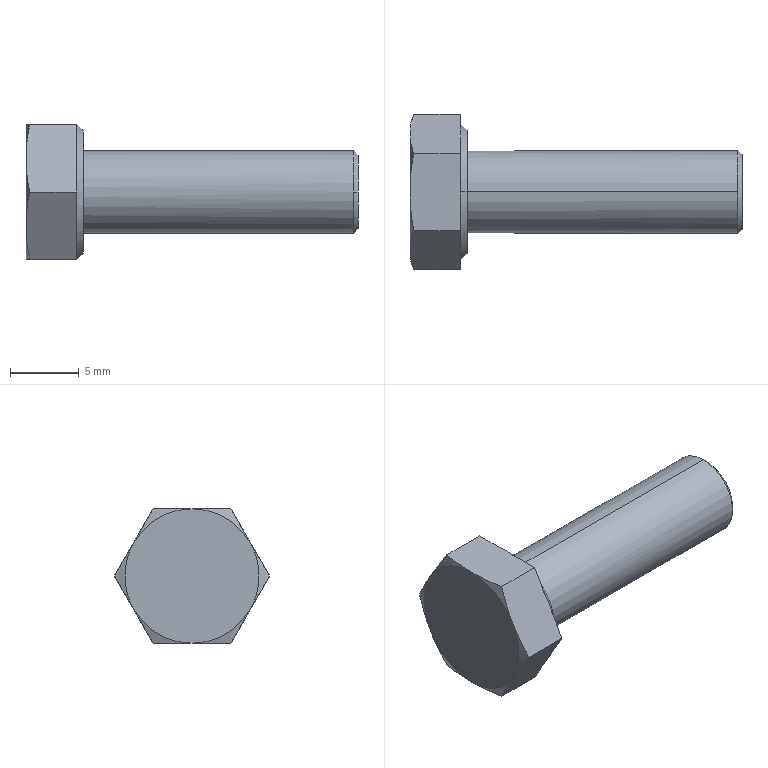Part | NX | features BREP 1 | 1 solid | 27 faces | box 24.15 x 11.293 x 9.78 mm | volume 900.954 mm3 | plane 15 | cone 10 | cylinder 2 | commonest cylinder face diameters 6 x2
STEP:
#1=CARTESIAN_POINT('',(0.,-4.235,-2.445));
#2=VERTEX_POINT('',#1);
#3=CARTESIAN_POINT('',(0.,0.,-4.89));
#4=VERTEX_POINT('',#3);
#5=CARTESIAN_POINT('',(0.,0.,0.));
#6=DIRECTION('',(1.,0.,0.));
#7=DIRECTION('',(0.,0.,-1.));
#8=AXIS2_PLACEMENT_3D('',#5,#6,#7);
#9=CIRCLE('',#8,4.89);
#10=EDGE_CURVE('',#2,#4,#9,.T.);
#11=ORIENTED_EDGE('',*,*,#10,.F.);
#12=CARTESIAN_POINT('',(0.,-4.235,2.445));
#13=VERTEX_POINT('',#12);
#14=CARTESIAN_POINT('',(0.,0.,0.));
#15=DIRECTION('',(1.,0.,0.));
#16=DIRECTION('',(0.,0.,-1.));
#17=AXIS2_PLACEMENT_3D('',#14,#15,#16);
#18=CIRCLE('',#17,4.89);
#19=EDGE_CURVE('',#13,#2,#18,.T.);
#20=ORIENTED_EDGE('',*,*,#19,.F.);
#21=CARTESIAN_POINT('',(0.,0.,4.89));
#22=VERTEX_POINT('',#21);
#23=CARTESIAN_POINT('',(0.,0.,0.));
#24=DIRECTION('',(1.,0.,0.));
#25=DIRECTION('',(0.,0.,-1.));
#26=AXIS2_PLACEMENT_3D('',#23,#24,#25);
#27=CIRCLE('',#26,4.89);
#28=EDGE_CURVE('',#22,#13,#27,.T.);
#29=ORIENTED_EDGE('',*,*,#28,.F.);
#30=CARTESIAN_POINT('',(0.,4.235,2.445));
#31=VERTEX_POINT('',#30);
#32=CARTESIAN_POINT('',(0.,0.,0.));
#33=DIRECTION('',(1.,0.,0.));
#34=DIRECTION('',(0.,0.,-1.));
#35=AXIS2_PLACEMENT_3D('',#32,#33,#34);
#36=CIRCLE('',#35,4.89);
#37=EDGE_CURVE('',#31,#22,#36,.T.);
#38=ORIENTED_EDGE('',*,*,#37,.F.);
#39=CARTESIAN_POINT('',(0.,4.235,-2.445));
#40=VERTEX_POINT('',#39);
#41=CARTESIAN_POINT('',(0.,0.,0.));
#42=DIRECTION('',(1.,0.,0.));
#43=DIRECTION('',(0.,0.,-1.));
#44=AXIS2_PLACEMENT_3D('',#41,#42,#43);
#45=CIRCLE('',#44,4.89);
#46=EDGE_CURVE('',#40,#31,#45,.T.);
#47=ORIENTED_EDGE('',*,*,#46,.F.);
#48=CARTESIAN_POINT('',(0.,0.,0.));
#49=DIRECTION('',(1.,0.,0.));
#50=DIRECTION('',(0.,0.,-1.));
#51=AXIS2_PLACEMENT_3D('',#48,#49,#50);
#52=CIRCLE('',#51,4.89);
#53=EDGE_CURVE('',#4,#40,#52,.T.);
#54=ORIENTED_EDGE('',*,*,#53,.F.);
#55=EDGE_LOOP('',(#11,#20,#29,#38,#47,#54));
#56=FACE_BOUND('',#55,.T.);
#57=CARTESIAN_POINT('',(0.,-2.823,-4.89));
#58=DIRECTION('',(1.,0.,0.));
#59=DIRECTION('',(0.,0.,-1.));
#60=AXIS2_PLACEMENT_3D('',#57,#58,#59);
#61=PLANE('',#60);
#62=ADVANCED_FACE('',(#56),#61,.F.);
#63=ORIENTED_EDGE('',*,*,#46,.T.);
#64=CARTESIAN_POINT('',(0.2753,5.646,0.));
#65=VERTEX_POINT('',#64);
#66=CARTESIAN_POINT('',(0.2753,5.646,0.));
#67=CARTESIAN_POINT('',(0.09178,5.142,0.8735));
#68=CARTESIAN_POINT('',(0.,4.672,1.689));
#69=CARTESIAN_POINT('',(0.,4.235,2.445));
#70=B_SPLINE_CURVE_WITH_KNOTS('',3,(#66,#67,#68,#69),.UNSPECIFIED.,.F.,.F.,(4,4),(0.,1.),.UNSPECIFIED.);
#71=EDGE_CURVE('',#31,#65,#70,.F.);
#72=ORIENTED_EDGE('',*,*,#71,.T.);
#73=CARTESIAN_POINT('',(0.,4.235,-2.445));
#74=CARTESIAN_POINT('',(0.,4.672,-1.689));
#75=CARTESIAN_POINT('',(0.09178,5.142,-0.8735));
#76=CARTESIAN_POINT('',(0.2753,5.646,0.));
#77=B_SPLINE_CURVE_WITH_KNOTS('',3,(#73,#74,#75,#76),.UNSPECIFIED.,.F.,.F.,(4,4),(0.,1.),.UNSPECIFIED.);
#78=EDGE_CURVE('',#65,#40,#77,.F.);
#79=ORIENTED_EDGE('',*,*,#78,.T.);
#80=EDGE_LOOP('',(#63,#72,#79));
#81=FACE_BOUND('',#80,.T.);
#82=CARTESIAN_POINT('',(0.277,0.,0.));
#83=DIRECTION('',(1.,0.,0.));
#84=DIRECTION('',(0.,0.,-1.));
#85=AXIS2_PLACEMENT_3D('',#82,#83,#84);
#86=CONICAL_SURFACE('',#85,5.651,1.222);
#87=ADVANCED_FACE('',(#81),#86,.T.);
#88=ORIENTED_EDGE('',*,*,#37,.T.);
#89=CARTESIAN_POINT('',(0.2753,2.823,4.89));
#90=VERTEX_POINT('',#89);
#91=CARTESIAN_POINT('',(0.2753,2.823,4.89));
#92=CARTESIAN_POINT('',(0.09178,1.815,4.89));
#93=CARTESIAN_POINT('',(0.,0.8735,4.89));
#94=CARTESIAN_POINT('',(0.,0.,4.89));
#95=B_SPLINE_CURVE_WITH_KNOTS('',3,(#91,#92,#93,#94),.UNSPECIFIED.,.F.,.F.,(4,4),(0.,1.),.UNSPECIFIED.);
#96=EDGE_CURVE('',#22,#90,#95,.F.);
#97=ORIENTED_EDGE('',*,*,#96,.T.);
#98=CARTESIAN_POINT('',(0.,4.235,2.445));
#99=CARTESIAN_POINT('',(0.,3.798,3.201));
#100=CARTESIAN_POINT('',(0.09178,3.328,4.016));
#101=CARTESIAN_POINT('',(0.2753,2.823,4.89));
#102=B_SPLINE_CURVE_WITH_KNOTS('',3,(#98,#99,#100,#101),.UNSPECIFIED.,.F.,.F.,(4,4),(0.,1.),.UNSPECIFIED.);
#103=EDGE_CURVE('',#90,#31,#102,.F.);
#104=ORIENTED_EDGE('',*,*,#103,.T.);
#105=EDGE_LOOP('',(#88,#97,#104));
#106=FACE_BOUND('',#105,.T.);
#107=CARTESIAN_POINT('',(0.277,0.,0.));
#108=DIRECTION('',(1.,0.,0.));
#109=DIRECTION('',(0.,0.,-1.));
#110=AXIS2_PLACEMENT_3D('',#107,#108,#109);
#111=CONICAL_SURFACE('',#110,5.651,1.222);
#112=ADVANCED_FACE('',(#106),#111,.T.);
#113=ORIENTED_EDGE('',*,*,#28,.T.);
#114=CARTESIAN_POINT('',(0.2753,-2.823,4.89));
#115=VERTEX_POINT('',#114);
#116=CARTESIAN_POINT('',(0.2753,-2.823,4.89));
#117=CARTESIAN_POINT('',(0.09178,-3.328,4.016));
#118=CARTESIAN_POINT('',(0.,-3.798,3.201));
#119=CARTESIAN_POINT('',(0.,-4.235,2.445));
#120=B_SPLINE_CURVE_WITH_KNOTS('',3,(#116,#117,#118,#119),.UNSPECIFIED.,.F.,.F.,(4,4),(0.,1.),.UNSPECIFIED.);
#121=EDGE_CURVE('',#13,#115,#120,.F.);
#122=ORIENTED_EDGE('',*,*,#121,.T.);
#123=CARTESIAN_POINT('',(0.,0.,4.89));
#124=CARTESIAN_POINT('',(0.,-0.8735,4.89));
#125=CARTESIAN_POINT('',(0.09178,-1.815,4.89));
#126=CARTESIAN_POINT('',(0.2753,-2.823,4.89));
#127=B_SPLINE_CURVE_WITH_KNOTS('',3,(#123,#124,#125,#126),.UNSPECIFIED.,.F.,.F.,(4,4),(0.,1.),.UNSPECIFIED.);
#128=EDGE_CURVE('',#115,#22,#127,.F.);
#129=ORIENTED_EDGE('',*,*,#128,.T.);
#130=EDGE_LOOP('',(#113,#122,#129));
#131=FACE_BOUND('',#130,.T.);
#132=CARTESIAN_POINT('',(0.277,0.,0.));
#133=DIRECTION('',(1.,0.,0.));
#134=DIRECTION('',(0.,0.,-1.));
#135=AXIS2_PLACEMENT_3D('',#132,#133,#134);
#136=CONICAL_SURFACE('',#135,5.651,1.222);
#137=ADVANCED_FACE('',(#131),#136,.T.);
#138=CARTESIAN_POINT('',(0.2753,-5.646,0.));
#139=VERTEX_POINT('',#138);
#140=CARTESIAN_POINT('',(0.,-4.235,2.445));
#141=CARTESIAN_POINT('',(0.,-4.672,1.689));
#142=CARTESIAN_POINT('',(0.09178,-5.142,0.8735));
#143=CARTESIAN_POINT('',(0.2753,-5.646,0.));
#144=B_SPLINE_CURVE_WITH_KNOTS('',3,(#140,#141,#142,#143),.UNSPECIFIED.,.F.,.F.,(4,4),(0.,1.),.UNSPECIFIED.);
#145=EDGE_CURVE('',#139,#13,#144,.F.);
#146=ORIENTED_EDGE('',*,*,#145,.T.);
#147=ORIENTED_EDGE('',*,*,#19,.T.);
#148=CARTESIAN_POINT('',(0.2753,-5.646,0.));
#149=CARTESIAN_POINT('',(0.09178,-5.142,-0.8735));
#150=CARTESIAN_POINT('',(0.,-4.672,-1.689));
#151=CARTESIAN_POINT('',(0.,-4.235,-2.445));
#152=B_SPLINE_CURVE_WITH_KNOTS('',3,(#148,#149,#150,#151),.UNSPECIFIED.,.F.,.F.,(4,4),(0.,1.),.UNSPECIFIED.);
#153=EDGE_CURVE('',#2,#139,#152,.F.);
#154=ORIENTED_EDGE('',*,*,#153,.T.);
#155=EDGE_LOOP('',(#146,#147,#154));
#156=FACE_BOUND('',#155,.T.);
#157=CARTESIAN_POINT('',(0.277,0.,0.));
#158=DIRECTION('',(1.,0.,0.));
#159=DIRECTION('',(0.,0.,-1.));
#160=AXIS2_PLACEMENT_3D('',#157,#158,#159);
#161=CONICAL_SURFACE('',#160,5.651,1.222);
#162=ADVANCED_FACE('',(#156),#161,.T.);
#163=CARTESIAN_POINT('',(0.2753,-2.823,-4.89));
#164=VERTEX_POINT('',#163);
#165=CARTESIAN_POINT('',(0.,-4.235,-2.445));
#166=CARTESIAN_POINT('',(0.,-3.798,-3.201));
#167=CARTESIAN_POINT('',(0.09178,-3.328,-4.016));
#168=CARTESIAN_POINT('',(0.2753,-2.823,-4.89));
#169=B_SPLINE_CURVE_WITH_KNOTS('',3,(#165,#166,#167,#168),.UNSPECIFIED.,.F.,.F.,(4,4),(0.,1.),.UNSPECIFIED.);
#170=EDGE_CURVE('',#164,#2,#169,.F.);
#171=ORIENTED_EDGE('',*,*,#170,.T.);
#172=ORIENTED_EDGE('',*,*,#10,.T.);
#173=CARTESIAN_POINT('',(0.2753,-2.823,-4.89));
#174=CARTESIAN_POINT('',(0.09178,-1.815,-4.89));
#175=CARTESIAN_POINT('',(0.,-0.8735,-4.89));
#176=CARTESIAN_POINT('',(0.,0.,-4.89));
#177=B_SPLINE_CURVE_WITH_KNOTS('',3,(#173,#174,#175,#176),.UNSPECIFIED.,.F.,.F.,(4,4),(0.,1.),.UNSPECIFIED.);
#178=EDGE_CURVE('',#4,#164,#177,.F.);
#179=ORIENTED_EDGE('',*,*,#178,.T.);
#180=EDGE_LOOP('',(#171,#172,#179));
#181=FACE_BOUND('',#180,.T.);
#182=CARTESIAN_POINT('',(0.277,0.,0.));
#183=DIRECTION('',(1.,0.,0.));
#184=DIRECTION('',(0.,0.,-1.));
#185=AXIS2_PLACEMENT_3D('',#182,#183,#184);
#186=CONICAL_SURFACE('',#185,5.651,1.222);
#187=ADVANCED_FACE('',(#181),#186,.T.);
#188=CARTESIAN_POINT('',(0.2753,2.823,-4.89));
#189=VERTEX_POINT('',#188);
#190=CARTESIAN_POINT('',(0.,0.,-4.89));
#191=CARTESIAN_POINT('',(0.,0.8735,-4.89));
#192=CARTESIAN_POINT('',(0.09178,1.815,-4.89));
#193=CARTESIAN_POINT('',(0.2753,2.823,-4.89));
#194=B_SPLINE_CURVE_WITH_KNOTS('',3,(#190,#191,#192,#193),.UNSPECIFIED.,.F.,.F.,(4,4),(0.,1.),.UNSPECIFIED.);
#195=EDGE_CURVE('',#189,#4,#194,.F.);
#196=ORIENTED_EDGE('',*,*,#195,.T.);
#197=ORIENTED_EDGE('',*,*,#53,.T.);
#198=CARTESIAN_POINT('',(0.2753,2.823,-4.89));
#199=CARTESIAN_POINT('',(0.09178,3.328,-4.016));
#200=CARTESIAN_POINT('',(0.,3.798,-3.201));
#201=CARTESIAN_POINT('',(0.,4.235,-2.445));
#202=B_SPLINE_CURVE_WITH_KNOTS('',3,(#198,#199,#200,#201),.UNSPECIFIED.,.F.,.F.,(4,4),(0.,1.),.UNSPECIFIED.);
#203=EDGE_CURVE('',#40,#189,#202,.F.);
#204=ORIENTED_EDGE('',*,*,#203,.T.);
#205=EDGE_LOOP('',(#196,#197,#204));
#206=FACE_BOUND('',#205,.T.);
#207=CARTESIAN_POINT('',(0.277,0.,0.));
#208=DIRECTION('',(1.,0.,0.));
#209=DIRECTION('',(0.,0.,-1.));
#210=AXIS2_PLACEMENT_3D('',#207,#208,#209);
#211=CONICAL_SURFACE('',#210,5.651,1.222);
#212=ADVANCED_FACE('',(#206),#211,.T.);
#213=CARTESIAN_POINT('',(3.65,2.823,-4.89));
#214=VERTEX_POINT('',#213);
#215=CARTESIAN_POINT('',(3.65,3.884,-3.052));
#216=VERTEX_POINT('',#215);
#217=CARTESIAN_POINT('',(3.65,2.823,-4.89));
#218=DIRECTION('',(0.,0.5,0.866));
#219=VECTOR('',#218,1000.);
#220=LINE('',#217,#219);
#221=EDGE_CURVE('',#214,#216,#220,.T.);
#222=ORIENTED_EDGE('',*,*,#221,.T.);
#223=CARTESIAN_POINT('',(3.65,0.7011,-4.89));
#224=VERTEX_POINT('',#223);
#225=CARTESIAN_POINT('',(3.65,0.,0.));
#226=DIRECTION('',(1.,0.,0.));
#227=DIRECTION('',(0.,0.,1.));
#228=AXIS2_PLACEMENT_3D('',#225,#226,#227);
#229=CIRCLE('',#228,4.94);
#230=EDGE_CURVE('',#224,#216,#229,.T.);
#231=ORIENTED_EDGE('',*,*,#230,.F.);
#232=CARTESIAN_POINT('',(3.65,-2.823,-4.89));
#233=DIRECTION('',(0.,1.,0.));
#234=VECTOR('',#233,1000.);
#235=LINE('',#232,#234);
#236=EDGE_CURVE('',#224,#214,#235,.T.);
#237=ORIENTED_EDGE('',*,*,#236,.T.);
#238=EDGE_LOOP('',(#222,#231,#237));
#239=FACE_BOUND('',#238,.T.);
#240=CARTESIAN_POINT('',(3.65,4.94,0.));
#241=DIRECTION('',(1.,0.,0.));
#242=DIRECTION('',(0.,0.,-1.));
#243=AXIS2_PLACEMENT_3D('',#240,#241,#242);
#244=PLANE('',#243);
#245=ADVANCED_FACE('',(#239),#244,.T.);
#246=CARTESIAN_POINT('',(3.65,5.646,0.));
#247=VERTEX_POINT('',#246);
#248=CARTESIAN_POINT('',(4.15,5.646,0.));
#249=DIRECTION('',(1.,0.,0.));
#250=VECTOR('',#249,1000.);
#251=LINE('',#248,#250);
#252=EDGE_CURVE('',#65,#247,#251,.T.);
#253=ORIENTED_EDGE('',*,*,#252,.T.);
#254=CARTESIAN_POINT('',(3.65,4.585,-1.838));
#255=VERTEX_POINT('',#254);
#256=CARTESIAN_POINT('',(3.65,4.585,-1.838));
#257=DIRECTION('',(0.,0.5,0.866));
#258=VECTOR('',#257,1000.);
#259=LINE('',#256,#258);
#260=EDGE_CURVE('',#255,#247,#259,.T.);
#261=ORIENTED_EDGE('',*,*,#260,.F.);
#262=CARTESIAN_POINT('',(3.65,4.585,-1.838));
#263=CARTESIAN_POINT('',(3.716,4.352,-2.243));
#264=CARTESIAN_POINT('',(3.716,4.118,-2.647));
#265=CARTESIAN_POINT('',(3.65,3.884,-3.052));
#266=B_SPLINE_CURVE_WITH_KNOTS('',3,(#262,#263,#264,#265),.UNSPECIFIED.,.F.,.F.,(4,4),(0.,1.),.UNSPECIFIED.);
#267=EDGE_CURVE('',#216,#255,#266,.F.);
#268=ORIENTED_EDGE('',*,*,#267,.F.);
#269=ORIENTED_EDGE('',*,*,#221,.F.);
#270=CARTESIAN_POINT('',(4.15,2.823,-4.89));
#271=DIRECTION('',(-1.,0.,0.));
#272=VECTOR('',#271,1000.);
#273=LINE('',#270,#272);
#274=EDGE_CURVE('',#214,#189,#273,.T.);
#275=ORIENTED_EDGE('',*,*,#274,.T.);
#276=ORIENTED_EDGE('',*,*,#203,.F.);
#277=ORIENTED_EDGE('',*,*,#78,.F.);
#278=EDGE_LOOP('',(#253,#261,#268,#269,#275,#276,#277));
#279=FACE_BOUND('',#278,.T.);
#280=CARTESIAN_POINT('',(4.15,2.823,-4.89));
#281=DIRECTION('',(0.,-0.866,0.5));
#282=DIRECTION('',(0.,-0.5,-0.866));
#283=AXIS2_PLACEMENT_3D('',#280,#281,#282);
#284=PLANE('',#283);
#285=ADVANCED_FACE('',(#279),#284,.F.);
#286=CARTESIAN_POINT('',(3.65,4.585,1.838));
#287=VERTEX_POINT('',#286);
#288=CARTESIAN_POINT('',(3.65,5.646,0.));
#289=DIRECTION('',(0.,-0.5,0.866));
#290=VECTOR('',#289,1000.);
#291=LINE('',#288,#290);
#292=EDGE_CURVE('',#247,#287,#291,.T.);
#293=ORIENTED_EDGE('',*,*,#292,.T.);
#294=CARTESIAN_POINT('',(3.65,0.,0.));
#295=DIRECTION('',(1.,0.,0.));
#296=DIRECTION('',(0.,0.,1.));
#297=AXIS2_PLACEMENT_3D('',#294,#295,#296);
#298=CIRCLE('',#297,4.94);
#299=EDGE_CURVE('',#255,#287,#298,.T.);
#300=ORIENTED_EDGE('',*,*,#299,.F.);
#301=ORIENTED_EDGE('',*,*,#260,.T.);
#302=EDGE_LOOP('',(#293,#300,#301));
#303=FACE_BOUND('',#302,.T.);
#304=CARTESIAN_POINT('',(3.65,4.94,0.));
#305=DIRECTION('',(1.,0.,0.));
#306=DIRECTION('',(0.,0.,-1.));
#307=AXIS2_PLACEMENT_3D('',#304,#305,#306);
#308=PLANE('',#307);
#309=ADVANCED_FACE('',(#303),#308,.T.);
#310=CARTESIAN_POINT('',(3.65,2.823,4.89));
#311=VERTEX_POINT('',#310);
#312=CARTESIAN_POINT('',(4.15,2.823,4.89));
#313=DIRECTION('',(1.,0.,0.));
#314=VECTOR('',#313,1000.);
#315=LINE('',#312,#314);
#316=EDGE_CURVE('',#90,#311,#315,.T.);
#317=ORIENTED_EDGE('',*,*,#316,.T.);
#318=CARTESIAN_POINT('',(3.65,3.884,3.052));
#319=VERTEX_POINT('',#318);
#320=CARTESIAN_POINT('',(3.65,3.884,3.052));
#321=DIRECTION('',(0.,-0.5,0.866));
#322=VECTOR('',#321,1000.);
#323=LINE('',#320,#322);
#324=EDGE_CURVE('',#319,#311,#323,.T.);
#325=ORIENTED_EDGE('',*,*,#324,.F.);
#326=CARTESIAN_POINT('',(3.65,3.884,3.052));
#327=CARTESIAN_POINT('',(3.716,4.118,2.647));
#328=CARTESIAN_POINT('',(3.716,4.352,2.243));
#329=CARTESIAN_POINT('',(3.65,4.585,1.838));
#330=B_SPLINE_CURVE_WITH_KNOTS('',3,(#326,#327,#328,#329),.UNSPECIFIED.,.F.,.F.,(4,4),(0.,1.),.UNSPECIFIED.);
#331=EDGE_CURVE('',#287,#319,#330,.F.);
#332=ORIENTED_EDGE('',*,*,#331,.F.);
#333=ORIENTED_EDGE('',*,*,#292,.F.);
#334=ORIENTED_EDGE('',*,*,#252,.F.);
#335=ORIENTED_EDGE('',*,*,#71,.F.);
#336=ORIENTED_EDGE('',*,*,#103,.F.);
#337=EDGE_LOOP('',(#317,#325,#332,#333,#334,#335,#336));
#338=FACE_BOUND('',#337,.T.);
#339=CARTESIAN_POINT('',(4.15,5.646,0.));
#340=DIRECTION('',(0.,-0.866,-0.5));
#341=DIRECTION('',(0.,0.5,-0.866));
#342=AXIS2_PLACEMENT_3D('',#339,#340,#341);
#343=PLANE('',#342);
#344=ADVANCED_FACE('',(#338),#343,.F.);
#345=CARTESIAN_POINT('',(3.65,0.7011,4.89));
#346=VERTEX_POINT('',#345);
#347=CARTESIAN_POINT('',(3.65,2.823,4.89));
#348=DIRECTION('',(0.,-1.,0.));
#349=VECTOR('',#348,1000.);
#350=LINE('',#347,#349);
#351=EDGE_CURVE('',#311,#346,#350,.T.);
#352=ORIENTED_EDGE('',*,*,#351,.T.);
#353=CARTESIAN_POINT('',(3.65,0.,0.));
#354=DIRECTION('',(1.,0.,0.));
#355=DIRECTION('',(0.,0.,1.));
#356=AXIS2_PLACEMENT_3D('',#353,#354,#355);
#357=CIRCLE('',#356,4.94);
#358=EDGE_CURVE('',#319,#346,#357,.T.);
#359=ORIENTED_EDGE('',*,*,#358,.F.);
#360=ORIENTED_EDGE('',*,*,#324,.T.);
#361=EDGE_LOOP('',(#352,#359,#360));
#362=FACE_BOUND('',#361,.T.);
#363=CARTESIAN_POINT('',(3.65,4.94,0.));
#364=DIRECTION('',(1.,0.,0.));
#365=DIRECTION('',(0.,0.,-1.));
#366=AXIS2_PLACEMENT_3D('',#363,#364,#365);
#367=PLANE('',#366);
#368=ADVANCED_FACE('',(#362),#367,.T.);
#369=CARTESIAN_POINT('',(3.65,-2.823,4.89));
#370=VERTEX_POINT('',#369);
#371=CARTESIAN_POINT('',(4.15,-2.823,4.89));
#372=DIRECTION('',(1.,0.,0.));
#373=VECTOR('',#372,1000.);
#374=LINE('',#371,#373);
#375=EDGE_CURVE('',#115,#370,#374,.T.);
#376=ORIENTED_EDGE('',*,*,#375,.T.);
#377=CARTESIAN_POINT('',(3.65,-0.7011,4.89));
#378=VERTEX_POINT('',#377);
#379=CARTESIAN_POINT('',(3.65,4.94,4.89));
#380=DIRECTION('',(0.,-1.,0.));
#381=VECTOR('',#380,1000.);
#382=LINE('',#379,#381);
#383=EDGE_CURVE('',#378,#370,#382,.T.);
#384=ORIENTED_EDGE('',*,*,#383,.F.);
#385=CARTESIAN_POINT('',(3.7,0.,4.89));
#386=VERTEX_POINT('',#385);
#387=CARTESIAN_POINT('',(3.65,-0.7011,4.89));
#388=CARTESIAN_POINT('',(3.683,-0.4662,4.89));
#389=CARTESIAN_POINT('',(3.7,-0.2325,4.89));
#390=CARTESIAN_POINT('',(3.7,0.,4.89));
#391=B_SPLINE_CURVE_WITH_KNOTS('',3,(#387,#388,#389,#390),.UNSPECIFIED.,.F.,.F.,(4,4),(0.,1.),.UNSPECIFIED.);
#392=EDGE_CURVE('',#386,#378,#391,.F.);
#393=ORIENTED_EDGE('',*,*,#392,.F.);
#394=CARTESIAN_POINT('',(3.7,0.,4.89));
#395=CARTESIAN_POINT('',(3.7,0.2325,4.89));
#396=CARTESIAN_POINT('',(3.683,0.4662,4.89));
#397=CARTESIAN_POINT('',(3.65,0.7011,4.89));
#398=B_SPLINE_CURVE_WITH_KNOTS('',3,(#394,#395,#396,#397),.UNSPECIFIED.,.F.,.F.,(4,4),(0.,1.),.UNSPECIFIED.);
#399=EDGE_CURVE('',#346,#386,#398,.F.);
#400=ORIENTED_EDGE('',*,*,#399,.F.);
#401=ORIENTED_EDGE('',*,*,#351,.F.);
#402=ORIENTED_EDGE('',*,*,#316,.F.);
#403=ORIENTED_EDGE('',*,*,#96,.F.);
#404=ORIENTED_EDGE('',*,*,#128,.F.);
#405=EDGE_LOOP('',(#376,#384,#393,#400,#401,#402,#403,#404));
#406=FACE_BOUND('',#405,.T.);
#407=CARTESIAN_POINT('',(4.15,2.823,4.89));
#408=DIRECTION('',(0.,0.,-1.));
#409=DIRECTION('',(-1.,0.,0.));
#410=AXIS2_PLACEMENT_3D('',#407,#408,#409);
#411=PLANE('',#410);
#412=ADVANCED_FACE('',(#406),#411,.F.);
#413=CARTESIAN_POINT('',(3.65,-3.884,3.052));
#414=VERTEX_POINT('',#413);
#415=CARTESIAN_POINT('',(3.65,-2.823,4.89));
#416=DIRECTION('',(0.,-0.5,-0.866));
#417=VECTOR('',#416,1000.);
#418=LINE('',#415,#417);
#419=EDGE_CURVE('',#370,#414,#418,.T.);
#420=ORIENTED_EDGE('',*,*,#419,.T.);
#421=CARTESIAN_POINT('',(3.65,0.,0.));
#422=DIRECTION('',(1.,0.,0.));
#423=DIRECTION('',(0.,0.,1.));
#424=AXIS2_PLACEMENT_3D('',#421,#422,#423);
#425=CIRCLE('',#424,4.94);
#426=EDGE_CURVE('',#378,#414,#425,.T.);
#427=ORIENTED_EDGE('',*,*,#426,.F.);
#428=ORIENTED_EDGE('',*,*,#383,.T.);
#429=EDGE_LOOP('',(#420,#427,#428));
#430=FACE_BOUND('',#429,.T.);
#431=CARTESIAN_POINT('',(3.65,4.94,0.));
#432=DIRECTION('',(1.,0.,0.));
#433=DIRECTION('',(0.,0.,-1.));
#434=AXIS2_PLACEMENT_3D('',#431,#432,#433);
#435=PLANE('',#434);
#436=ADVANCED_FACE('',(#430),#435,.T.);
#437=CARTESIAN_POINT('',(3.65,-5.646,0.));
#438=VERTEX_POINT('',#437);
#439=CARTESIAN_POINT('',(4.15,-5.646,0.));
#440=DIRECTION('',(1.,0.,0.));
#441=VECTOR('',#440,1000.);
#442=LINE('',#439,#441);
#443=EDGE_CURVE('',#139,#438,#442,.T.);
#444=ORIENTED_EDGE('',*,*,#443,.T.);
#445=CARTESIAN_POINT('',(3.65,-4.585,1.838));
#446=VERTEX_POINT('',#445);
#447=CARTESIAN_POINT('',(3.65,-4.585,1.838));
#448=DIRECTION('',(0.,-0.5,-0.866));
#449=VECTOR('',#448,1000.);
#450=LINE('',#447,#449);
#451=EDGE_CURVE('',#446,#438,#450,.T.);
#452=ORIENTED_EDGE('',*,*,#451,.F.);
#453=CARTESIAN_POINT('',(3.65,-4.585,1.838));
#454=CARTESIAN_POINT('',(3.716,-4.352,2.243));
#455=CARTESIAN_POINT('',(3.716,-4.118,2.647));
#456=CARTESIAN_POINT('',(3.65,-3.884,3.052));
#457=B_SPLINE_CURVE_WITH_KNOTS('',3,(#453,#454,#455,#456),.UNSPECIFIED.,.F.,.F.,(4,4),(0.,1.),.UNSPECIFIED.);
#458=EDGE_CURVE('',#414,#446,#457,.F.);
#459=ORIENTED_EDGE('',*,*,#458,.F.);
#460=ORIENTED_EDGE('',*,*,#419,.F.);
#461=ORIENTED_EDGE('',*,*,#375,.F.);
#462=ORIENTED_EDGE('',*,*,#121,.F.);
#463=ORIENTED_EDGE('',*,*,#145,.F.);
#464=EDGE_LOOP('',(#444,#452,#459,#460,#461,#462,#463));
#465=FACE_BOUND('',#464,.T.);
#466=CARTESIAN_POINT('',(4.15,-2.823,4.89));
#467=DIRECTION('',(0.,0.866,-0.5));
#468=DIRECTION('',(0.,0.5,0.866));
#469=AXIS2_PLACEMENT_3D('',#466,#467,#468);
#470=PLANE('',#469);
#471=ADVANCED_FACE('',(#465),#470,.F.);
#472=CARTESIAN_POINT('',(3.65,-4.585,-1.838));
#473=VERTEX_POINT('',#472);
#474=CARTESIAN_POINT('',(3.65,0.,0.));
#475=DIRECTION('',(1.,0.,0.));
#476=DIRECTION('',(0.,0.,1.));
#477=AXIS2_PLACEMENT_3D('',#474,#475,#476);
#478=CIRCLE('',#477,4.94);
#479=EDGE_CURVE('',#446,#473,#478,.T.);
#480=ORIENTED_EDGE('',*,*,#479,.F.);
#481=ORIENTED_EDGE('',*,*,#451,.T.);
#482=CARTESIAN_POINT('',(3.65,-5.646,0.));
#483=DIRECTION('',(0.,0.5,-0.866));
#484=VECTOR('',#483,1000.);
#485=LINE('',#482,#484);
#486=EDGE_CURVE('',#438,#473,#485,.T.);
#487=ORIENTED_EDGE('',*,*,#486,.T.);
#488=EDGE_LOOP('',(#480,#481,#487));
#489=FACE_BOUND('',#488,.T.);
#490=CARTESIAN_POINT('',(3.65,4.94,0.));
#491=DIRECTION('',(1.,0.,0.));
#492=DIRECTION('',(0.,0.,-1.));
#493=AXIS2_PLACEMENT_3D('',#490,#491,#492);
#494=PLANE('',#493);
#495=ADVANCED_FACE('',(#489),#494,.T.);
#496=CARTESIAN_POINT('',(3.65,-2.823,-4.89));
#497=VERTEX_POINT('',#496);
#498=CARTESIAN_POINT('',(4.15,-2.823,-4.89));
#499=DIRECTION('',(1.,0.,0.));
#500=VECTOR('',#499,1000.);
#501=LINE('',#498,#500);
#502=EDGE_CURVE('',#164,#497,#501,.T.);
#503=ORIENTED_EDGE('',*,*,#502,.T.);
#504=CARTESIAN_POINT('',(3.65,-3.884,-3.052));
#505=VERTEX_POINT('',#504);
#506=CARTESIAN_POINT('',(3.65,-3.884,-3.052));
#507=DIRECTION('',(0.,0.5,-0.866));
#508=VECTOR('',#507,1000.);
#509=LINE('',#506,#508);
#510=EDGE_CURVE('',#505,#497,#509,.T.);
#511=ORIENTED_EDGE('',*,*,#510,.F.);
#512=CARTESIAN_POINT('',(3.65,-3.884,-3.052));
#513=CARTESIAN_POINT('',(3.716,-4.118,-2.647));
#514=CARTESIAN_POINT('',(3.716,-4.352,-2.243));
#515=CARTESIAN_POINT('',(3.65,-4.585,-1.838));
#516=B_SPLINE_CURVE_WITH_KNOTS('',3,(#512,#513,#514,#515),.UNSPECIFIED.,.F.,.F.,(4,4),(0.,1.),.UNSPECIFIED.);
#517=EDGE_CURVE('',#473,#505,#516,.F.);
#518=ORIENTED_EDGE('',*,*,#517,.F.);
#519=ORIENTED_EDGE('',*,*,#486,.F.);
#520=ORIENTED_EDGE('',*,*,#443,.F.);
#521=ORIENTED_EDGE('',*,*,#153,.F.);
#522=ORIENTED_EDGE('',*,*,#170,.F.);
#523=EDGE_LOOP('',(#503,#511,#518,#519,#520,#521,#522));
#524=FACE_BOUND('',#523,.T.);
#525=CARTESIAN_POINT('',(4.15,-5.646,0.));
#526=DIRECTION('',(0.,0.866,0.5));
#527=DIRECTION('',(0.,-0.5,0.866));
#528=AXIS2_PLACEMENT_3D('',#525,#526,#527);
#529=PLANE('',#528);
#530=ADVANCED_FACE('',(#524),#529,.F.);
#531=CARTESIAN_POINT('',(3.65,-0.7011,-4.89));
#532=VERTEX_POINT('',#531);
#533=CARTESIAN_POINT('',(3.65,-2.823,-4.89));
#534=DIRECTION('',(0.,1.,0.));
#535=VECTOR('',#534,1000.);
#536=LINE('',#533,#535);
#537=EDGE_CURVE('',#497,#532,#536,.T.);
#538=ORIENTED_EDGE('',*,*,#537,.T.);
#539=CARTESIAN_POINT('',(3.65,0.,0.));
#540=DIRECTION('',(1.,0.,0.));
#541=DIRECTION('',(0.,0.,1.));
#542=AXIS2_PLACEMENT_3D('',#539,#540,#541);
#543=CIRCLE('',#542,4.94);
#544=EDGE_CURVE('',#505,#532,#543,.T.);
#545=ORIENTED_EDGE('',*,*,#544,.F.);
#546=ORIENTED_EDGE('',*,*,#510,.T.);
#547=EDGE_LOOP('',(#538,#545,#546));
#548=FACE_BOUND('',#547,.T.);
#549=CARTESIAN_POINT('',(3.65,4.94,0.));
#550=DIRECTION('',(1.,0.,0.));
#551=DIRECTION('',(0.,0.,-1.));
#552=AXIS2_PLACEMENT_3D('',#549,#550,#551);
#553=PLANE('',#552);
#554=ADVANCED_FACE('',(#548),#553,.T.);
#555=ORIENTED_EDGE('',*,*,#274,.F.);
#556=ORIENTED_EDGE('',*,*,#236,.F.);
#557=CARTESIAN_POINT('',(3.7,0.,-4.89));
#558=VERTEX_POINT('',#557);
#559=CARTESIAN_POINT('',(3.65,0.7011,-4.89));
#560=CARTESIAN_POINT('',(3.683,0.4662,-4.89));
#561=CARTESIAN_POINT('',(3.7,0.2325,-4.89));
#562=CARTESIAN_POINT('',(3.7,0.,-4.89));
#563=B_SPLINE_CURVE_WITH_KNOTS('',3,(#559,#560,#561,#562),.UNSPECIFIED.,.F.,.F.,(4,4),(0.,1.),.UNSPECIFIED.);
#564=EDGE_CURVE('',#558,#224,#563,.F.);
#565=ORIENTED_EDGE('',*,*,#564,.F.);
#566=CARTESIAN_POINT('',(3.7,0.,-4.89));
#567=CARTESIAN_POINT('',(3.7,-0.2325,-4.89));
#568=CARTESIAN_POINT('',(3.683,-0.4662,-4.89));
#569=CARTESIAN_POINT('',(3.65,-0.7011,-4.89));
#570=B_SPLINE_CURVE_WITH_KNOTS('',3,(#566,#567,#568,#569),.UNSPECIFIED.,.F.,.F.,(4,4),(0.,1.),.UNSPECIFIED.);
#571=EDGE_CURVE('',#532,#558,#570,.F.);
#572=ORIENTED_EDGE('',*,*,#571,.F.);
#573=ORIENTED_EDGE('',*,*,#537,.F.);
#574=ORIENTED_EDGE('',*,*,#502,.F.);
#575=ORIENTED_EDGE('',*,*,#178,.F.);
#576=ORIENTED_EDGE('',*,*,#195,.F.);
#577=EDGE_LOOP('',(#555,#556,#565,#572,#573,#574,#575,#576));
#578=FACE_BOUND('',#577,.T.);
#579=CARTESIAN_POINT('',(4.15,-2.823,-4.89));
#580=DIRECTION('',(0.,0.,1.));
#581=DIRECTION('',(0.,-1.,0.));
#582=AXIS2_PLACEMENT_3D('',#579,#580,#581);
#583=PLANE('',#582);
#584=ADVANCED_FACE('',(#578),#583,.F.);
#585=CARTESIAN_POINT('',(24.15,-2.7,0.));
#586=VERTEX_POINT('',#585);
#587=CARTESIAN_POINT('',(24.15,2.7,0.));
#588=VERTEX_POINT('',#587);
#589=CARTESIAN_POINT('',(24.15,0.,0.));
#590=DIRECTION('',(-1.,0.,0.));
#591=DIRECTION('',(0.,-1.,0.));
#592=AXIS2_PLACEMENT_3D('',#589,#590,#591);
#593=CIRCLE('',#592,2.7);
#594=EDGE_CURVE('',#586,#588,#593,.T.);
#595=ORIENTED_EDGE('',*,*,#594,.F.);
#596=CARTESIAN_POINT('',(24.15,0.,0.));
#597=DIRECTION('',(-1.,0.,0.));
#598=DIRECTION('',(0.,-1.,0.));
#599=AXIS2_PLACEMENT_3D('',#596,#597,#598);
#600=CIRCLE('',#599,2.7);
#601=EDGE_CURVE('',#588,#586,#600,.T.);
#602=ORIENTED_EDGE('',*,*,#601,.F.);
#603=EDGE_LOOP('',(#595,#602));
#604=FACE_BOUND('',#603,.T.);
#605=CARTESIAN_POINT('',(24.15,0.,0.));
#606=DIRECTION('',(1.,0.,0.));
#607=DIRECTION('',(0.,0.,-1.));
#608=AXIS2_PLACEMENT_3D('',#605,#606,#607);
#609=PLANE('',#608);
#610=ADVANCED_FACE('',(#604),#609,.T.);
#611=CARTESIAN_POINT('',(4.15,0.,-4.44));
#612=VERTEX_POINT('',#611);
#613=CARTESIAN_POINT('',(3.65,0.,-4.94));
#614=DIRECTION('',(-0.7071,0.,-0.7071));
#615=VECTOR('',#614,1000.);
#616=LINE('',#613,#615);
#617=EDGE_CURVE('',#558,#612,#616,.F.);
#618=ORIENTED_EDGE('',*,*,#617,.T.);
#619=CARTESIAN_POINT('',(4.15,0.,4.44));
#620=VERTEX_POINT('',#619);
#621=CARTESIAN_POINT('',(4.15,0.,0.));
#622=DIRECTION('',(1.,0.,0.));
#623=DIRECTION('',(0.,0.,1.));
#624=AXIS2_PLACEMENT_3D('',#621,#622,#623);
#625=CIRCLE('',#624,4.44);
#626=EDGE_CURVE('',#620,#612,#625,.T.);
#627=ORIENTED_EDGE('',*,*,#626,.F.);
#628=CARTESIAN_POINT('',(3.65,0.,4.94));
#629=DIRECTION('',(-0.7071,0.,0.7071));
#630=VECTOR('',#629,1000.);
#631=LINE('',#628,#630);
#632=EDGE_CURVE('',#386,#620,#631,.F.);
#633=ORIENTED_EDGE('',*,*,#632,.F.);
#634=ORIENTED_EDGE('',*,*,#392,.T.);
#635=ORIENTED_EDGE('',*,*,#426,.T.);
#636=ORIENTED_EDGE('',*,*,#458,.T.);
#637=ORIENTED_EDGE('',*,*,#479,.T.);
#638=ORIENTED_EDGE('',*,*,#517,.T.);
#639=ORIENTED_EDGE('',*,*,#544,.T.);
#640=ORIENTED_EDGE('',*,*,#571,.T.);
#641=EDGE_LOOP('',(#618,#627,#633,#634,#635,#636,#637,#638,#639,#640));
#642=FACE_BOUND('',#641,.T.);
#643=CARTESIAN_POINT('',(3.65,0.,0.));
#644=DIRECTION('',(-1.,0.,0.));
#645=DIRECTION('',(0.,0.,1.));
#646=AXIS2_PLACEMENT_3D('',#643,#644,#645);
#647=CONICAL_SURFACE('',#646,4.94,0.7854);
#648=ADVANCED_FACE('',(#642),#647,.T.);
#649=CARTESIAN_POINT('',(23.85,3.,0.));
#650=VERTEX_POINT('',#649);
#651=CARTESIAN_POINT('',(23.85,3.,0.));
#652=DIRECTION('',(-0.7071,0.7071,0.));
#653=VECTOR('',#652,1000.);
#654=LINE('',#651,#653);
#655=EDGE_CURVE('',#588,#650,#654,.T.);
#656=ORIENTED_EDGE('',*,*,#655,.F.);
#657=ORIENTED_EDGE('',*,*,#601,.T.);
#658=CARTESIAN_POINT('',(23.85,-3.,0.));
#659=VERTEX_POINT('',#658);
#660=CARTESIAN_POINT('',(23.85,-3.,0.));
#661=DIRECTION('',(-0.7071,-0.7071,0.));
#662=VECTOR('',#661,1000.);
#663=LINE('',#660,#662);
#664=EDGE_CURVE('',#586,#659,#663,.T.);
#665=ORIENTED_EDGE('',*,*,#664,.T.);
#666=CARTESIAN_POINT('',(23.85,0.,-3.));
#667=VERTEX_POINT('',#666);
#668=CARTESIAN_POINT('',(23.85,0.,0.));
#669=DIRECTION('',(-1.,0.,0.));
#670=DIRECTION('',(0.,0.,1.));
#671=AXIS2_PLACEMENT_3D('',#668,#669,#670);
#672=CIRCLE('',#671,3.);
#673=EDGE_CURVE('',#667,#659,#672,.T.);
#674=ORIENTED_EDGE('',*,*,#673,.F.);
#675=CARTESIAN_POINT('',(23.85,0.,0.));
#676=DIRECTION('',(-1.,0.,0.));
#677=DIRECTION('',(0.,0.,1.));
#678=AXIS2_PLACEMENT_3D('',#675,#676,#677);
#679=CIRCLE('',#678,3.);
#680=EDGE_CURVE('',#650,#667,#679,.T.);
#681=ORIENTED_EDGE('',*,*,#680,.F.);
#682=EDGE_LOOP('',(#656,#657,#665,#674,#681));
#683=FACE_BOUND('',#682,.T.);
#684=CARTESIAN_POINT('',(23.85,0.,0.));
#685=DIRECTION('',(-1.,0.,0.));
#686=DIRECTION('',(0.,-1.,0.));
#687=AXIS2_PLACEMENT_3D('',#684,#685,#686);
#688=CONICAL_SURFACE('',#687,3.,0.7854);
#689=ADVANCED_FACE('',(#683),#688,.T.);
#690=ORIENTED_EDGE('',*,*,#626,.T.);
#691=CARTESIAN_POINT('',(4.15,0.,0.));
#692=DIRECTION('',(1.,0.,0.));
#693=DIRECTION('',(0.,0.,1.));
#694=AXIS2_PLACEMENT_3D('',#691,#692,#693);
#695=CIRCLE('',#694,4.44);
#696=EDGE_CURVE('',#612,#620,#695,.T.);
#697=ORIENTED_EDGE('',*,*,#696,.T.);
#698=EDGE_LOOP('',(#690,#697));
#699=FACE_BOUND('',#698,.T.);
#700=CARTESIAN_POINT('',(4.15,0.,3.));
#701=VERTEX_POINT('',#700);
#702=CARTESIAN_POINT('',(4.15,0.,-3.));
#703=VERTEX_POINT('',#702);
#704=CARTESIAN_POINT('',(4.15,0.,0.));
#705=DIRECTION('',(1.,0.,0.));
#706=DIRECTION('',(0.,0.,1.));
#707=AXIS2_PLACEMENT_3D('',#704,#705,#706);
#708=CIRCLE('',#707,3.);
#709=EDGE_CURVE('',#701,#703,#708,.T.);
#710=ORIENTED_EDGE('',*,*,#709,.F.);
#711=CARTESIAN_POINT('',(4.15,0.,0.));
#712=DIRECTION('',(1.,0.,0.));
#713=DIRECTION('',(0.,0.,1.));
#714=AXIS2_PLACEMENT_3D('',#711,#712,#713);
#715=CIRCLE('',#714,3.);
#716=EDGE_CURVE('',#703,#701,#715,.T.);
#717=ORIENTED_EDGE('',*,*,#716,.F.);
#718=EDGE_LOOP('',(#710,#717));
#719=FACE_BOUND('',#718,.T.);
#720=CARTESIAN_POINT('',(4.15,-2.823,-4.89));
#721=DIRECTION('',(1.,0.,0.));
#722=DIRECTION('',(0.,0.,-1.));
#723=AXIS2_PLACEMENT_3D('',#720,#721,#722);
#724=PLANE('',#723);
#725=ADVANCED_FACE('',(#699,#719),#724,.T.);
#726=CARTESIAN_POINT('',(24.15,0.,-3.));
#727=DIRECTION('',(-1.,0.,0.));
#728=VECTOR('',#727,1000.);
#729=LINE('',#726,#728);
#730=EDGE_CURVE('',#703,#667,#729,.F.);
#731=ORIENTED_EDGE('',*,*,#730,.T.);
#732=ORIENTED_EDGE('',*,*,#673,.T.);
#733=CARTESIAN_POINT('',(23.85,0.,3.));
#734=VERTEX_POINT('',#733);
#735=CARTESIAN_POINT('',(23.85,0.,0.));
#736=DIRECTION('',(-1.,0.,0.));
#737=DIRECTION('',(0.,0.,1.));
#738=AXIS2_PLACEMENT_3D('',#735,#736,#737);
#739=CIRCLE('',#738,3.);
#740=EDGE_CURVE('',#659,#734,#739,.T.);
#741=ORIENTED_EDGE('',*,*,#740,.T.);
#742=CARTESIAN_POINT('',(24.15,0.,3.));
#743=DIRECTION('',(-1.,0.,0.));
#744=VECTOR('',#743,1000.);
#745=LINE('',#742,#744);
#746=EDGE_CURVE('',#701,#734,#745,.F.);
#747=ORIENTED_EDGE('',*,*,#746,.F.);
#748=ORIENTED_EDGE('',*,*,#709,.T.);
#749=EDGE_LOOP('',(#731,#732,#741,#747,#748));
#750=FACE_BOUND('',#749,.T.);
#751=CARTESIAN_POINT('',(24.15,0.,0.));
#752=DIRECTION('',(-1.,0.,0.));
#753=DIRECTION('',(0.,0.,1.));
#754=AXIS2_PLACEMENT_3D('',#751,#752,#753);
#755=CYLINDRICAL_SURFACE('',#754,3.);
#756=ADVANCED_FACE('',(#750),#755,.T.);
#757=ORIENTED_EDGE('',*,*,#696,.F.);
#758=ORIENTED_EDGE('',*,*,#617,.F.);
#759=ORIENTED_EDGE('',*,*,#564,.T.);
#760=ORIENTED_EDGE('',*,*,#230,.T.);
#761=ORIENTED_EDGE('',*,*,#267,.T.);
#762=ORIENTED_EDGE('',*,*,#299,.T.);
#763=ORIENTED_EDGE('',*,*,#331,.T.);
#764=ORIENTED_EDGE('',*,*,#358,.T.);
#765=ORIENTED_EDGE('',*,*,#399,.T.);
#766=ORIENTED_EDGE('',*,*,#632,.T.);
#767=EDGE_LOOP('',(#757,#758,#759,#760,#761,#762,#763,#764,#765,#766));
#768=FACE_BOUND('',#767,.T.);
#769=CARTESIAN_POINT('',(3.65,0.,0.));
#770=DIRECTION('',(-1.,0.,0.));
#771=DIRECTION('',(0.,0.,1.));
#772=AXIS2_PLACEMENT_3D('',#769,#770,#771);
#773=CONICAL_SURFACE('',#772,4.94,0.7854);
#774=ADVANCED_FACE('',(#768),#773,.T.);
#775=ORIENTED_EDGE('',*,*,#594,.T.);
#776=ORIENTED_EDGE('',*,*,#655,.T.);
#777=CARTESIAN_POINT('',(23.85,0.,0.));
#778=DIRECTION('',(-1.,0.,0.));
#779=DIRECTION('',(0.,0.,1.));
#780=AXIS2_PLACEMENT_3D('',#777,#778,#779);
#781=CIRCLE('',#780,3.);
#782=EDGE_CURVE('',#734,#650,#781,.T.);
#783=ORIENTED_EDGE('',*,*,#782,.F.);
#784=ORIENTED_EDGE('',*,*,#740,.F.);
#785=ORIENTED_EDGE('',*,*,#664,.F.);
#786=EDGE_LOOP('',(#775,#776,#783,#784,#785));
#787=FACE_BOUND('',#786,.T.);
#788=CARTESIAN_POINT('',(23.85,0.,0.));
#789=DIRECTION('',(-1.,0.,0.));
#790=DIRECTION('',(0.,-1.,0.));
#791=AXIS2_PLACEMENT_3D('',#788,#789,#790);
#792=CONICAL_SURFACE('',#791,3.,0.7854);
#793=ADVANCED_FACE('',(#787),#792,.T.);
#794=ORIENTED_EDGE('',*,*,#680,.T.);
#795=ORIENTED_EDGE('',*,*,#730,.F.);
#796=ORIENTED_EDGE('',*,*,#716,.T.);
#797=ORIENTED_EDGE('',*,*,#746,.T.);
#798=ORIENTED_EDGE('',*,*,#782,.T.);
#799=EDGE_LOOP('',(#794,#795,#796,#797,#798));
#800=FACE_BOUND('',#799,.T.);
#801=CARTESIAN_POINT('',(24.15,0.,0.));
#802=DIRECTION('',(-1.,0.,0.));
#803=DIRECTION('',(0.,0.,1.));
#804=AXIS2_PLACEMENT_3D('',#801,#802,#803);
#805=CYLINDRICAL_SURFACE('',#804,3.);
#806=ADVANCED_FACE('',(#800),#805,.T.);
#807=CLOSED_SHELL('',(#62,#87,#112,#137,#162,#187,#212,#245,#285,#309,#344,#368,#412,#436,#471,#495,#530,#554,#584,#610,#648,#689,#725,#756,#774,#793,#806));
#808=MANIFOLD_SOLID_BREP('',#807);
#809=(LENGTH_UNIT()NAMED_UNIT(*)SI_UNIT(.MILLI.,.METRE.));
#810=UNCERTAINTY_MEASURE_WITH_UNIT(LENGTH_MEASURE(0.0508),#809,'','');
#811=(NAMED_UNIT(*)PLANE_ANGLE_UNIT()SI_UNIT($,.RADIAN.));
#812=(NAMED_UNIT(*)SI_UNIT($,.STERADIAN.)SOLID_ANGLE_UNIT());
#813=(GEOMETRIC_REPRESENTATION_CONTEXT(3)GLOBAL_UNCERTAINTY_ASSIGNED_CONTEXT((#810))GLOBAL_UNIT_ASSIGNED_CONTEXT((#809,#811,#812))REPRESENTATION_CONTEXT('',''));
#814=ADVANCED_BREP_SHAPE_REPRESENTATION('',(#808),#813);